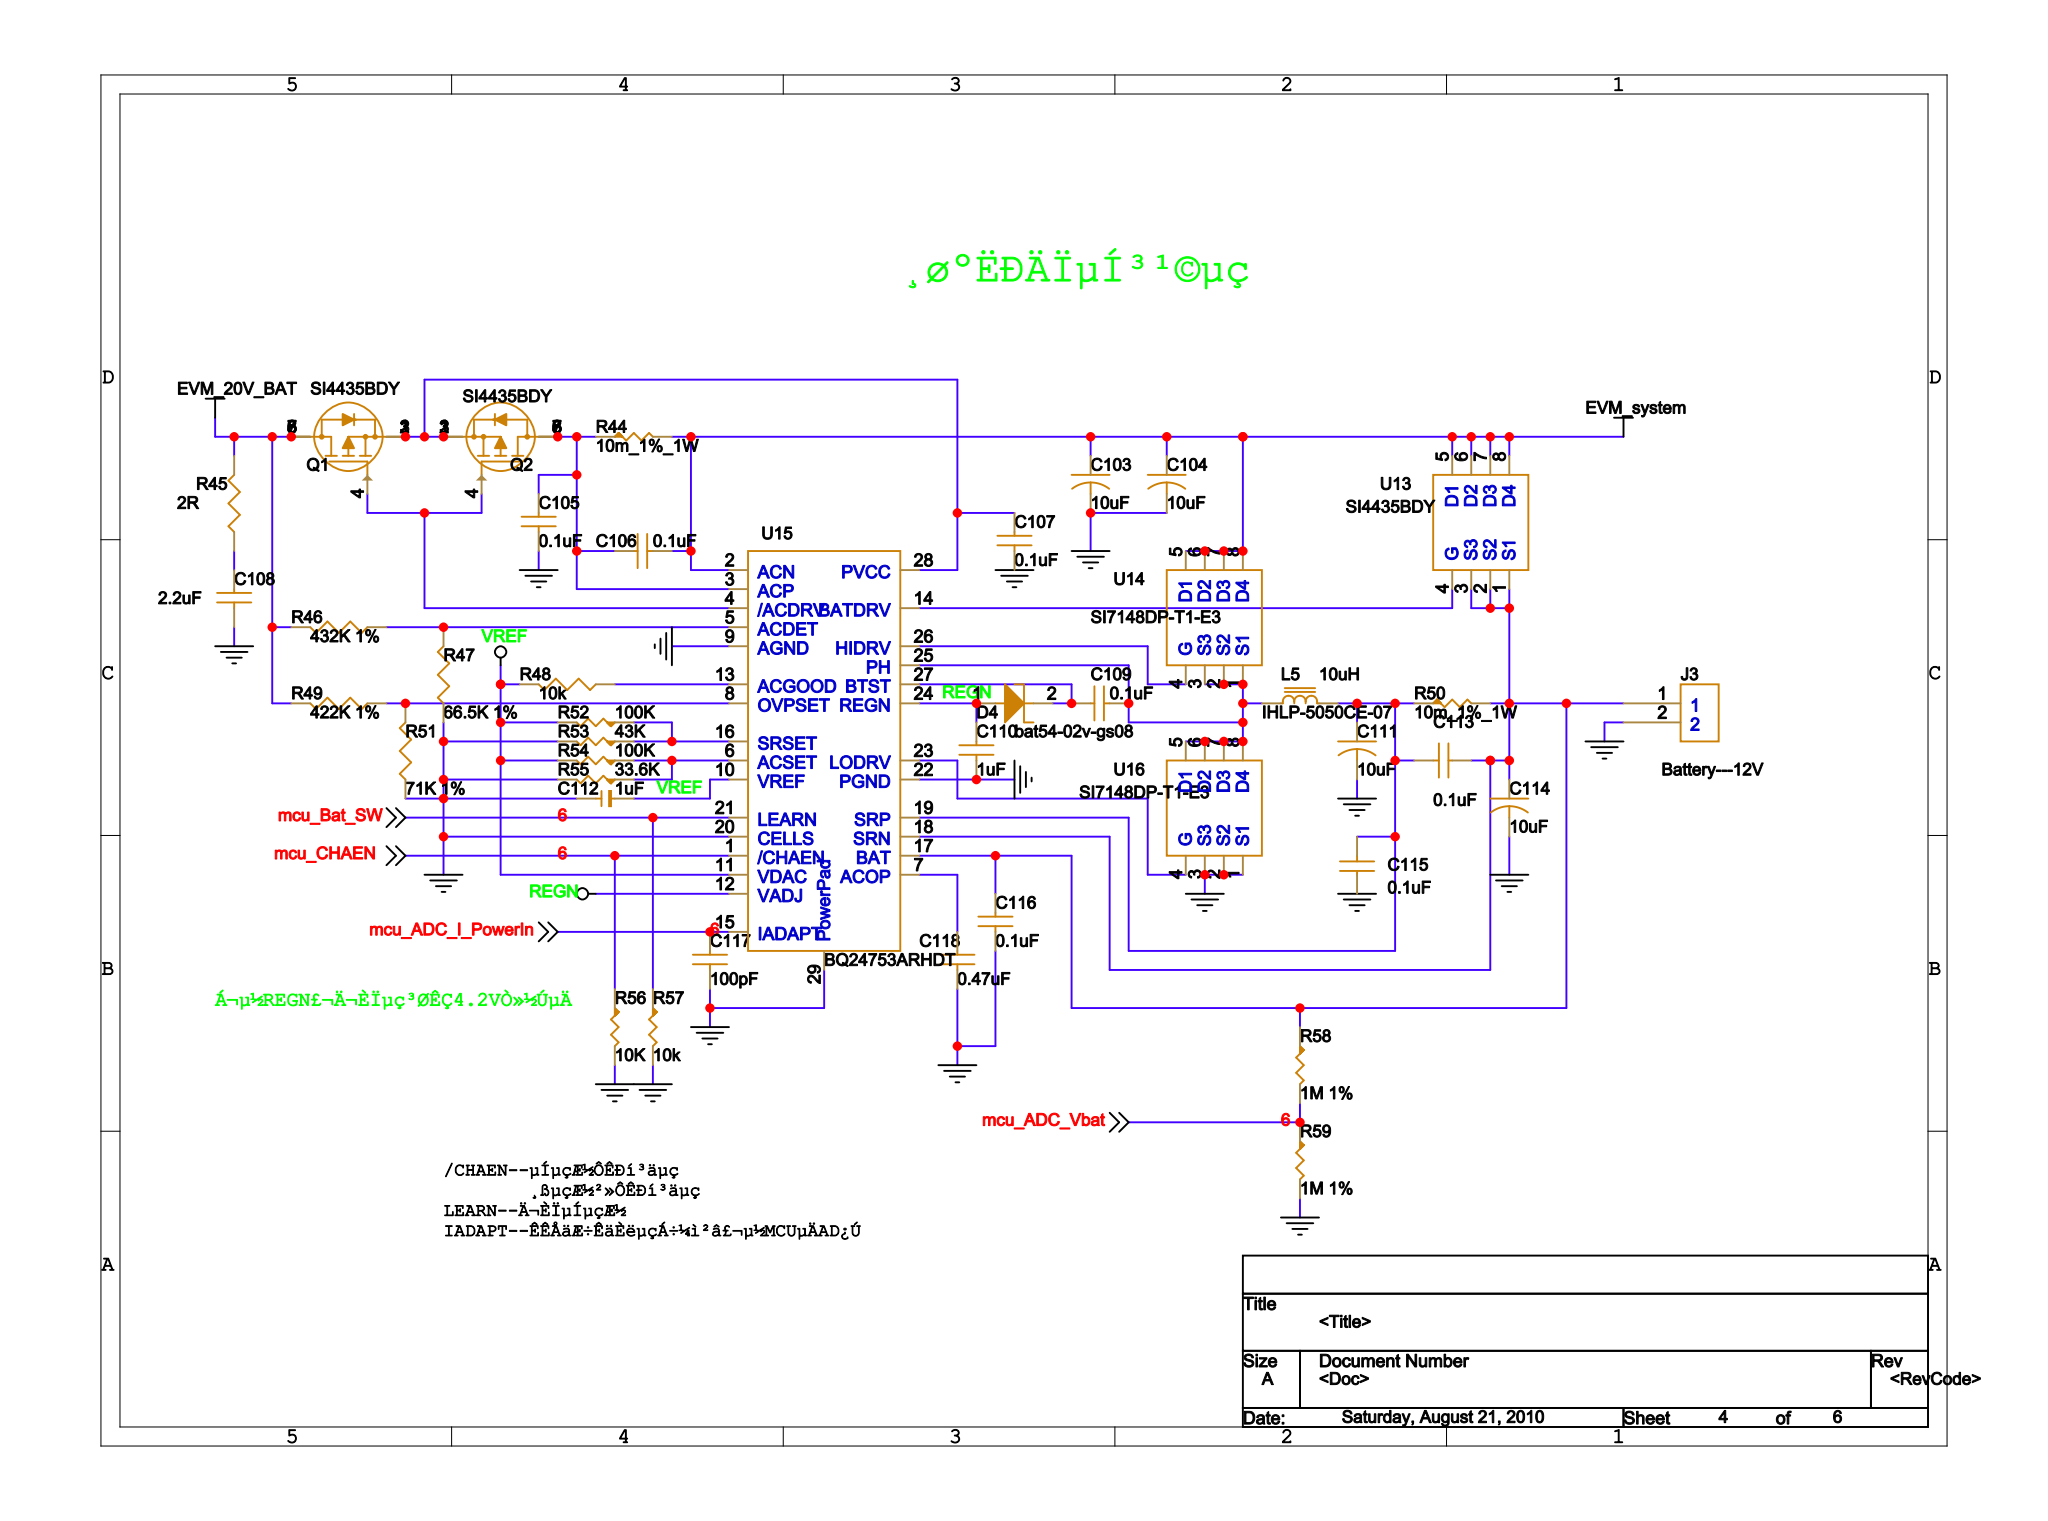Circuit board | Cadence Allegro | 241 parts | 116 nets | one sheet of the schematic
Parts on this sheet (reference | value | footprint):
C103 | 10uF | C1210
C104 | 10uF | C1210
C105 | 0.1uF | R0603
C106 | 0.1uF | R0603
C107 | 0.1uF | C0603
C108 | 2.2uF | C0603
C109 | 0.1uF | C0603
C110 | 1uF | C0603
C111 | 10uF | C1210
C112 | 1uF | C0603
C113 | 0.1uF | C0603
C114 | 10uF | C1210
C115 | 0.1uF | C0603
C116 | 0.1uF | C0603
C117 | 100pF | C0603
C118 | 0.47uF | C0603
D4 | bat54-02v-gs08 | SOD_523
J3 | Battery---12V | HDR2MM54_1X2
L5 | 10uH | L-12X12X7
Q1 | SI4435BDY | SO_8_PAD
Q2 | SI4435BDY | SO_8_PAD
R44 | 10m_1%_1W | R1206
R45 | 2R | R0603
R46 | 432K 1% | R0603
R47 | 66.5K 1% | R0603
R48 | 10K | R0603
R49 | 422K 1% | R0603
R50 | 10m_1%_1W | R1206
R51 | 71K 1% | R0603
R52 | 100K | R0603
R53 | 43K | R0603
R54 | 100K | R0603
R55 | 33.6K | R0603
R56 | 10K | R0603
R57 | 10K | R0603
R58 | 1M 1% | R0603
R59 | 1M 1% | R0603
U13 | SI4435BDY | SO_8_PAD
U14 | SI7148DP-T1-E3 | SO_8_PAD
U15 | BQ24753ARHDT | QFN28
U16 | SI7148DP-T1-E3 | SO_8_PAD
Nets of these parts (net: part-pin ...):
EVM_SYSTEM: C103-1 C104-1 C106-2 R44-2 U13-5 U13-6 U13-7 U13-8 U14-5 U14-6 U14-7 U14-8 U15-2
GND: C103-2 C104-2 C105-2 C107-2 C108-2 C110-2 C111-2 C112-1 C114-2 C115-1 C116-2 C117-2 C118-2 J3-2 R47-1 R51-1 R53-2 R55-2 R56-2 R57-2 R59-2 U16-1 U16-2 U16-3 U15-9 U15-20 U15-22 U15-29
N19167326: C107-1 Q1-1 Q1-2 Q1-3 Q2-1 Q2-2 Q2-3 U15-28
N19167882: C109-1 D4-2 U15-27
N19167213: C109-2 L5-1 U14-1 U14-2 U14-3 U16-5 U16-6 U16-7 U16-8 U15-25
N19167201: C113-1 C114-1 C116-1 J3-1 R50-2 R58-1 U13-1 U13-2 U13-3 U15-17 U15-18
N19167246: C111-1 C113-2 C115-2 L5-2 R50-1 U15-19
N19167205: C105-1 C106-1 Q2-5 Q2-6 Q2-7 Q2-8 R44-1 U15-3
EVM_20V_BAT: Q1-5 Q1-6 Q1-7 Q1-8 R45-2 R46-2 R49-2
VREF: C112-2 R48-2 R52-2 R54-2 U15-10 U15-11
MCU_ADC_I_POWERIN: C117-1 U15-15
N19167784: C118-1 U15-7
N19167580: R48-1 U15-13
MCU_ADC_VBAT: R58-2 R59-1
N19167554: C108-1 R45-1
N19167418: R46-1 R47-2 U15-5
N19167460: R49-1 R51-2 U15-8
N19167195: R52-1 R53-1 U15-16
N19167197: R54-1 R55-1 U15-6
MCU_CHAEN: R56-1 U15-1
MCU_BAT_SW: R57-1 U15-21
N19167550: U13-4 U15-14
REGN: C110-1 D4-1 U15-12 U15-24
N19167330: Q1-4 Q2-4 U15-4
N19167856: U14-4 U15-26
N19167909: U16-4 U15-23